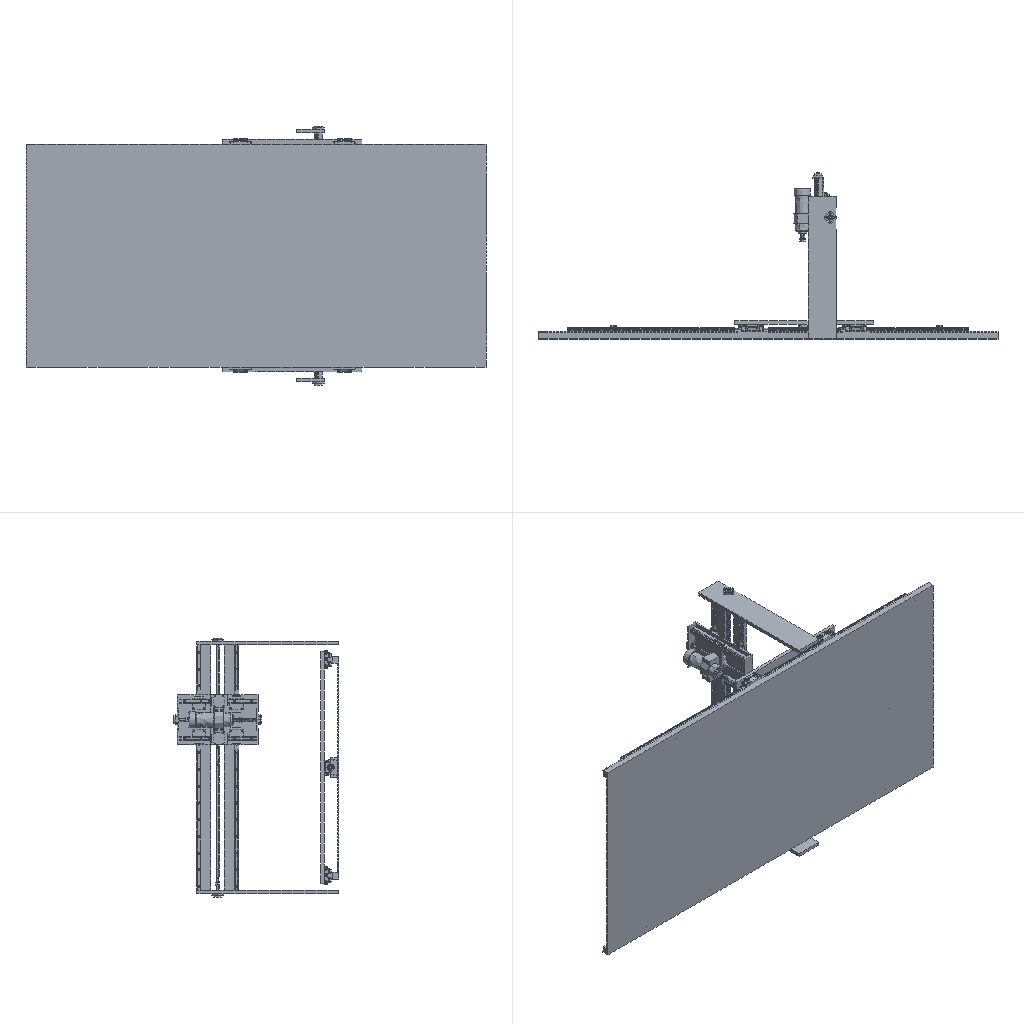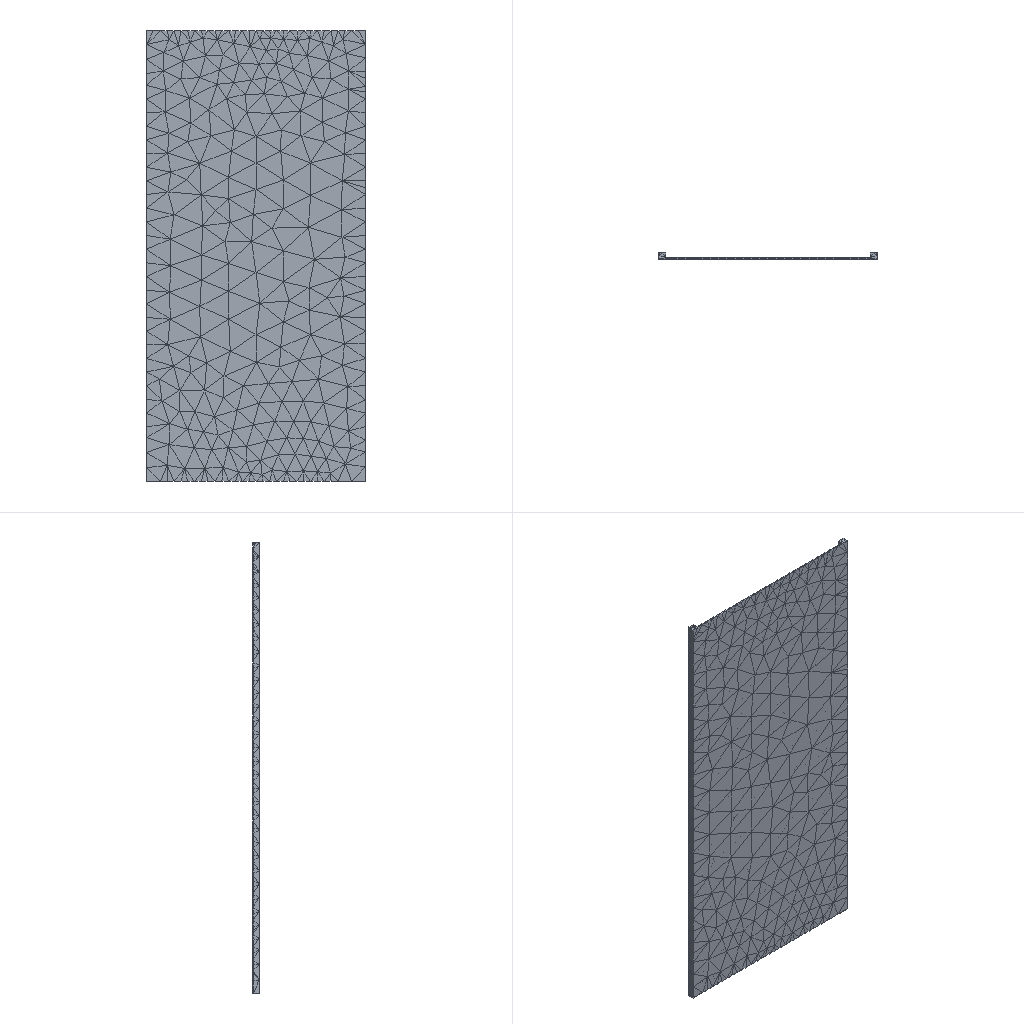Simulation study | ansys workbench
Set-up summary, first 217 of 1033 lines:
category,name,step,type,value,unit,region
solver,ansys_mapdl
solver,version,,,22.1
solver,version,,,22.1
units,MPA,,stated
analysis,deck1,,static,static
load_step,requested,,,1
analysis,nlgeom,,,False
mesh,nodes,,,7701
mesh,elements,,,4419
element_type,ANSYS 187 (type 1),,solid,3637
element_type,ANSYS 154 (type 2),,surface,782
load,load commands in deck,,count,3
bc,support commands in deck,,count,1
named_set,_FIXEDSU,,component
analysis,deck2,,static,static
load_step,requested,,,1
analysis,nlgeom,,,False
mesh,nodes,,,409419
mesh,elements,,,337105
element_type,ANSYS 187 (type 1),,solid,1852
element_type,ANSYS 187 (type 2),,solid,2828
element_type,ANSYS 186 (type 3),,solid,12
element_type,ANSYS 186 (type 4),,solid,12
element_type,ANSYS 187 (type 5),,solid,6973
element_type,ANSYS 187 (type 6),,solid,2227
element_type,ANSYS 187 (type 7),,solid,2227
element_type,ANSYS 187 (type 8),,solid,796
element_type,ANSYS 187 (type 9),,solid,283
element_type,ANSYS 187 (type 10),,solid,283
element_type,ANSYS 187 (type 11),,solid,283
element_type,ANSYS 187 (type 12),,solid,283
element_type,ANSYS 187 (type 13),,solid,217
element_type,ANSYS 187 (type 14),,solid,6973
element_type,ANSYS 187 (type 15),,solid,2227
element_type,ANSYS 187 (type 16),,solid,2227
element_type,ANSYS 187 (type 17),,solid,796
element_type,ANSYS 187 (type 18),,solid,283
element_type,ANSYS 187 (type 19),,solid,283
element_type,ANSYS 187 (type 20),,solid,283
element_type,ANSYS 187 (type 21),,solid,283
element_type,ANSYS 187 (type 22),,solid,217
element_type,ANSYS 187 (type 23),,solid,10177
element_type,ANSYS 187 (type 24),,solid,6973
element_type,ANSYS 187 (type 25),,solid,2227
element_type,ANSYS 187 (type 26),,solid,2227
element_type,ANSYS 187 (type 27),,solid,796
element_type,ANSYS 187 (type 28),,solid,283
element_type,ANSYS 187 (type 29),,solid,283
element_type,ANSYS 187 (type 30),,solid,283
element_type,ANSYS 187 (type 31),,solid,283
element_type,ANSYS 187 (type 32),,solid,217
element_type,ANSYS 187 (type 33),,solid,6973
element_type,ANSYS 187 (type 34),,solid,2227
element_type,ANSYS 187 (type 35),,solid,2227
element_type,ANSYS 187 (type 36),,solid,796
element_type,ANSYS 187 (type 37),,solid,283
element_type,ANSYS 187 (type 38),,solid,283
element_type,ANSYS 187 (type 39),,solid,283
element_type,ANSYS 187 (type 40),,solid,283
element_type,ANSYS 187 (type 41),,solid,217
element_type,ANSYS 187 (type 42),,solid,10177
element_type,ANSYS 187 (type 43),,solid,2654
element_type,ANSYS 186 (type 44),,solid,12
element_type,ANSYS 186 (type 45),,solid,12
element_type,ANSYS 187 (type 46),,solid,5788
element_type,ANSYS 187 (type 47),,solid,1456
element_type,ANSYS 187 (type 48),,solid,1456
element_type,ANSYS 187 (type 49),,solid,258
element_type,ANSYS 187 (type 50),,solid,283
element_type,ANSYS 187 (type 51),,solid,283
element_type,ANSYS 187 (type 52),,solid,283
element_type,ANSYS 187 (type 53),,solid,283
element_type,ANSYS 187 (type 54),,solid,235
element_type,ANSYS 187 (type 55),,solid,5788
element_type,ANSYS 187 (type 56),,solid,1456
element_type,ANSYS 187 (type 57),,solid,1456
element_type,ANSYS 187 (type 58),,solid,258
element_type,ANSYS 187 (type 59),,solid,283
element_type,ANSYS 187 (type 60),,solid,283
element_type,ANSYS 187 (type 61),,solid,283
element_type,ANSYS 187 (type 62),,solid,283
element_type,ANSYS 187 (type 63),,solid,235
element_type,ANSYS 187 (type 64),,solid,9433
element_type,ANSYS 187 (type 65),,solid,5788
element_type,ANSYS 187 (type 66),,solid,1456
element_type,ANSYS 187 (type 67),,solid,1456
element_type,ANSYS 187 (type 68),,solid,258
element_type,ANSYS 187 (type 69),,solid,283
element_type,ANSYS 187 (type 70),,solid,283
element_type,ANSYS 187 (type 71),,solid,283
element_type,ANSYS 187 (type 72),,solid,283
element_type,ANSYS 187 (type 73),,solid,235
element_type,ANSYS 187 (type 74),,solid,5788
element_type,ANSYS 187 (type 75),,solid,1456
element_type,ANSYS 187 (type 76),,solid,1456
element_type,ANSYS 187 (type 77),,solid,258
element_type,ANSYS 187 (type 78),,solid,283
element_type,ANSYS 187 (type 79),,solid,283
element_type,ANSYS 187 (type 80),,solid,283
element_type,ANSYS 187 (type 81),,solid,283
element_type,ANSYS 187 (type 82),,solid,235
element_type,ANSYS 187 (type 83),,solid,9433
element_type,ANSYS 186 (type 84),,solid,132
element_type,ANSYS 186 (type 85),,solid,132
element_type,ANSYS 186 (type 86),,solid,136
element_type,ANSYS 186 (type 87),,solid,136
element_type,ANSYS 187 (type 88),,solid,770
element_type,ANSYS 187 (type 89),,solid,1278
element_type,ANSYS 187 (type 90),,solid,1278
element_type,ANSYS 187 (type 91),,solid,770
element_type,ANSYS 187 (type 92),,solid,1373
element_type,ANSYS 187 (type 93),,solid,214
element_type,ANSYS 187 (type 94),,solid,5788
element_type,ANSYS 187 (type 95),,solid,1456
element_type,ANSYS 187 (type 96),,solid,1456
element_type,ANSYS 187 (type 97),,solid,258
element_type,ANSYS 187 (type 98),,solid,283
element_type,ANSYS 187 (type 99),,solid,283
element_type,ANSYS 187 (type 100),,solid,283
element_type,ANSYS 187 (type 101),,solid,283
element_type,ANSYS 187 (type 102),,solid,235
element_type,ANSYS 187 (type 103),,solid,3327
element_type,ANSYS 187 (type 104),,solid,5788
element_type,ANSYS 187 (type 105),,solid,1456
element_type,ANSYS 187 (type 106),,solid,1456
element_type,ANSYS 187 (type 107),,solid,258
element_type,ANSYS 187 (type 108),,solid,283
element_type,ANSYS 187 (type 109),,solid,283
element_type,ANSYS 187 (type 110),,solid,283
element_type,ANSYS 187 (type 111),,solid,283
element_type,ANSYS 187 (type 112),,solid,235
element_type,ANSYS 187 (type 113),,solid,3327
element_type,ANSYS 187 (type 114),,solid,2654
element_type,ANSYS 186 (type 115),,solid,12
element_type,ANSYS 186 (type 116),,solid,12
element_type,ANSYS 187 (type 117),,solid,1209
element_type,ANSYS 187 (type 118),,solid,770
element_type,ANSYS 187 (type 119),,solid,770
element_type,ANSYS 187 (type 120),,solid,1278
element_type,ANSYS 187 (type 121),,solid,1278
element_type,ANSYS 187 (type 122),,solid,2756
element_type,ANSYS 187 (type 123),,solid,214
element_type,ANSYS 186 (type 124),,solid,36
element_type,ANSYS 187 (type 125),,solid,13177
element_type,ANSYS 187 (type 126),,solid,1745
element_type,ANSYS 187 (type 127),,solid,1445
element_type,ANSYS 187 (type 128),,solid,1745
element_type,ANSYS 187 (type 129),,solid,1445
element_type,ANSYS 186 (type 130),,solid,1050
element_type,ANSYS 186 (type 131),,solid,17
element_type,ANSYS 187 (type 132),,solid,1999
element_type,ANSYS 187 (type 133),,solid,4031
element_type,ANSYS 174 (type 134),,contact,112
element_type,ANSYS 170 (type 135),,target,112
element_type,ANSYS 174 (type 136),,contact,42
element_type,ANSYS 170 (type 137),,target,42
element_type,ANSYS 174 (type 138),,contact,36
element_type,ANSYS 170 (type 139),,target,36
element_type,ANSYS 174 (type 140),,contact,250
element_type,ANSYS 170 (type 141),,target,250
element_type,ANSYS 174 (type 142),,contact,246
element_type,ANSYS 170 (type 143),,target,246
element_type,ANSYS 174 (type 144),,contact,60
element_type,ANSYS 170 (type 145),,target,60
element_type,ANSYS 174 (type 146),,contact,60
element_type,ANSYS 170 (type 147),,target,60
element_type,ANSYS 174 (type 148),,contact,433
element_type,ANSYS 170 (type 149),,target,433
element_type,ANSYS 174 (type 150),,contact,295
element_type,ANSYS 170 (type 151),,target,295
element_type,ANSYS 174 (type 152),,contact,292
element_type,ANSYS 170 (type 153),,target,292
element_type,ANSYS 174 (type 154),,contact,200
element_type,ANSYS 170 (type 155),,target,200
element_type,ANSYS 174 (type 156),,contact,186
element_type,ANSYS 170 (type 157),,target,186
element_type,ANSYS 174 (type 158),,contact,183
element_type,ANSYS 170 (type 159),,target,183
element_type,ANSYS 174 (type 160),,contact,187
element_type,ANSYS 170 (type 161),,target,187
element_type,ANSYS 174 (type 162),,contact,186
element_type,ANSYS 170 (type 163),,target,186
element_type,ANSYS 174 (type 164),,contact,204
element_type,ANSYS 170 (type 165),,target,204
element_type,ANSYS 174 (type 166),,contact,409
element_type,ANSYS 170 (type 167),,target,409
element_type,ANSYS 174 (type 168),,contact,95
element_type,ANSYS 170 (type 169),,target,95
element_type,ANSYS 174 (type 170),,contact,216
element_type,ANSYS 170 (type 171),,target,216
element_type,ANSYS 174 (type 172),,contact,194
element_type,ANSYS 170 (type 173),,target,194
element_type,ANSYS 174 (type 174),,contact,202
element_type,ANSYS 170 (type 175),,target,202
element_type,ANSYS 174 (type 176),,contact,92
element_type,ANSYS 170 (type 177),,target,92
element_type,ANSYS 174 (type 178),,contact,232
element_type,ANSYS 170 (type 179),,target,232
element_type,ANSYS 174 (type 180),,contact,34
element_type,ANSYS 170 (type 181),,target,34
element_type,ANSYS 174 (type 182),,contact,20
element_type,ANSYS 170 (type 183),,target,20
element_type,ANSYS 174 (type 184),,contact,225
element_type,ANSYS 170 (type 185),,target,225
element_type,ANSYS 174 (type 186),,contact,194
element_type,ANSYS 170 (type 187),,target,194
element_type,ANSYS 174 (type 188),,contact,202
element_type,ANSYS 170 (type 189),,target,202
element_type,ANSYS 174 (type 190),,contact,235
element_type,ANSYS 170 (type 191),,target,235
element_type,ANSYS 174 (type 192),,contact,30
element_type,ANSYS 170 (type 193),,target,30
element_type,ANSYS 174 (type 194),,contact,20
element_type,ANSYS 170 (type 195),,target,20
element_type,ANSYS 174 (type 196),,contact,45
element_type,ANSYS 170 (type 197),,target,45
Results summary:
result,analysis,,,static
result,last_loadstep,,,1
result,primary field,,,displacement
result,reaction total,1,FX,0.0,N
result,reaction total,1,FY,499999999.995,N
result,reaction total,1,FZ,0.0,N
result,mass,,,0.0632,"NMM: mm, ton, N, s, mV, mA, degC"
result,analysis,,,static
result,last_loadstep,,,1
result,primary field,,,displacement
result,reaction total,1,FX,-1e-06,N
result,reaction total,1,FY,5000000,N
result,reaction total,1,FZ,-0.000121,N
result,mass,,,0.149,"NMM: mm, ton, N, s, mV, mA, degC"